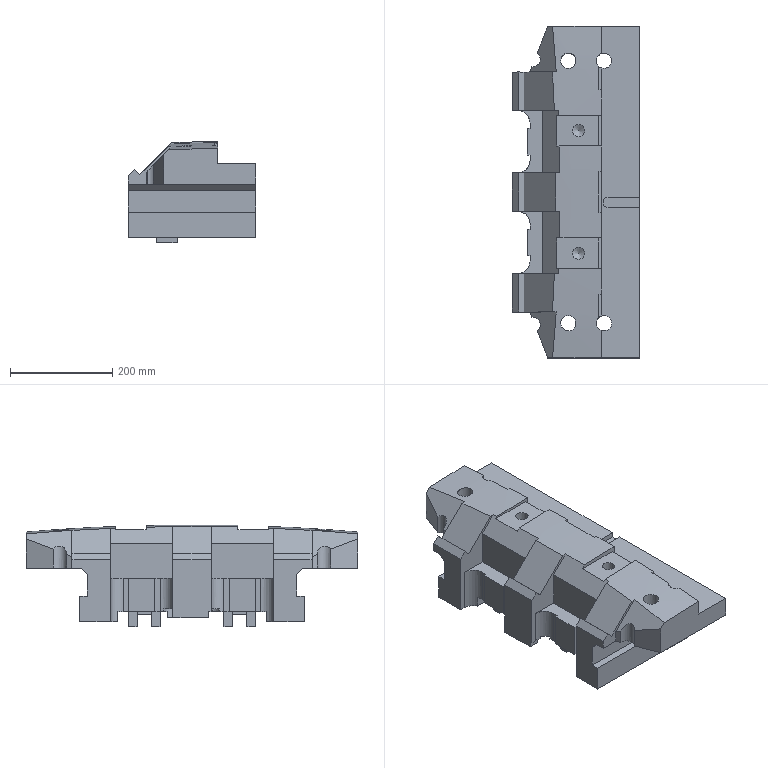Part | NX | features MAIN_BODY 2 | 1 solid | 165 faces | box 250 x 650 x 199.214 mm | volume 15663327 mm3 | plane 139 | cylinder 21 | spline 3 | cone 2 | commonest cylinder face diameters 30 x10 50 x4 24 x2 40 x2 42 x2 20 x1